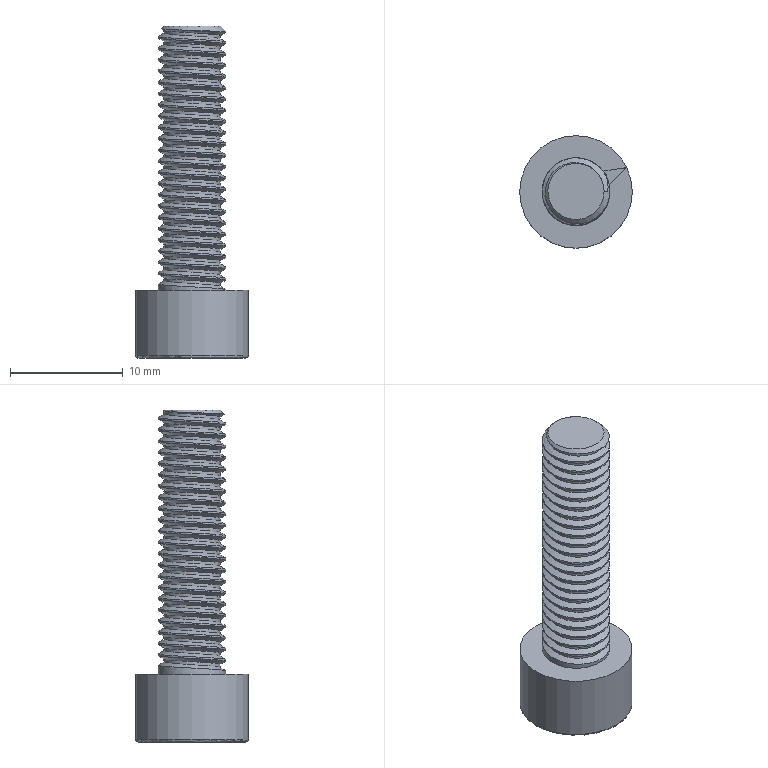Part | STEP file | Tube feed_id122_x_t | 1 solid | 26 faces | box 10 x 10 x 29.5 mm | volume 938.206 mm3 | plane 12 | cylinder 9 | spline 3 | cone 1 | torus 1 | commonest cylinder face diameters 0.4 x6 5 x1 6 x1 10 x1